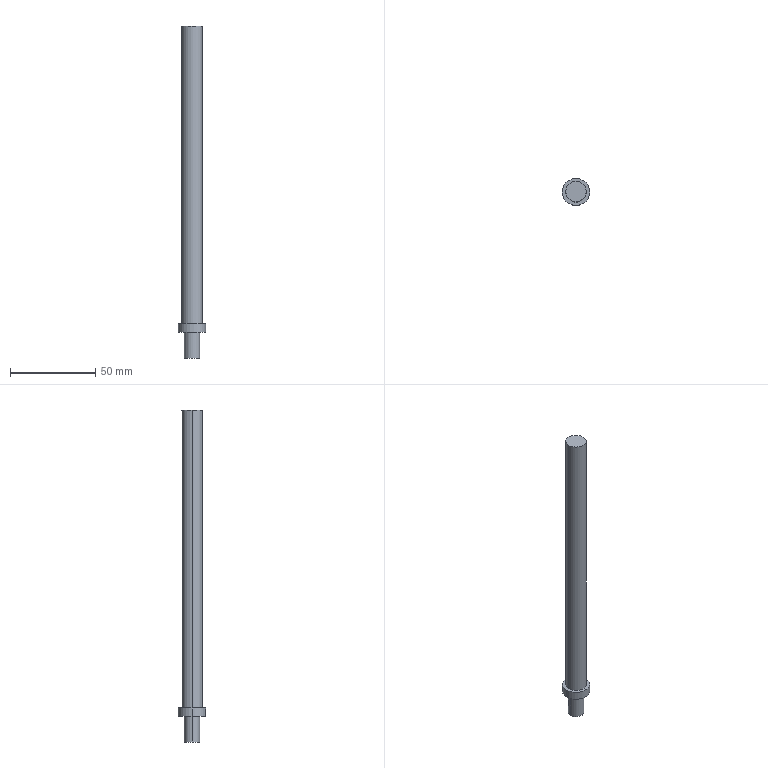Part | SolidWorks | features ICE 2, Extrusion 1 | 1 solid | 10 faces | box 16 x 16 x 195 mm | volume 21752 mm3 | cylinder 6 | plane 4 | commonest cylinder face diameters 9 x2 12 x2 16 x2
STEP:
#1=CARTESIAN_POINT('',(6.,0.,195.));
#2=VERTEX_POINT('',#1);
#3=CARTESIAN_POINT('',(-6.,0.,195.));
#4=VERTEX_POINT('',#3);
#5=CARTESIAN_POINT('',(0.,0.,195.));
#6=DIRECTION('',(0.,0.,1.));
#7=DIRECTION('',(1.,0.,0.));
#8=AXIS2_PLACEMENT_3D('',#5,#6,#7);
#9=CIRCLE('',#8,6.);
#10=EDGE_CURVE('',#2,#4,#9,.T.);
#11=ORIENTED_EDGE('',*,*,#10,.F.);
#12=CARTESIAN_POINT('',(6.,0.,20.));
#13=VERTEX_POINT('',#12);
#14=CARTESIAN_POINT('',(6.,0.,195.));
#15=DIRECTION('',(0.,0.,-1.));
#16=VECTOR('',#15,1000.);
#17=LINE('',#14,#16);
#18=EDGE_CURVE('',#2,#13,#17,.T.);
#19=ORIENTED_EDGE('',*,*,#18,.T.);
#20=CARTESIAN_POINT('',(-6.,0.,20.));
#21=VERTEX_POINT('',#20);
#22=CARTESIAN_POINT('',(0.,0.,20.));
#23=DIRECTION('',(0.,0.,-1.));
#24=DIRECTION('',(-1.,0.,0.));
#25=AXIS2_PLACEMENT_3D('',#22,#23,#24);
#26=CIRCLE('',#25,6.);
#27=EDGE_CURVE('',#21,#13,#26,.T.);
#28=ORIENTED_EDGE('',*,*,#27,.F.);
#29=CARTESIAN_POINT('',(-6.,0.,195.));
#30=DIRECTION('',(0.,0.,-1.));
#31=VECTOR('',#30,1000.);
#32=LINE('',#29,#31);
#33=EDGE_CURVE('',#4,#21,#32,.T.);
#34=ORIENTED_EDGE('',*,*,#33,.F.);
#35=EDGE_LOOP('',(#11,#19,#28,#34));
#36=FACE_OUTER_BOUND('',#35,.T.);
#37=CARTESIAN_POINT('',(0.,0.,195.));
#38=DIRECTION('',(0.,0.,-1.));
#39=DIRECTION('',(-1.,0.,0.));
#40=AXIS2_PLACEMENT_3D('',#37,#38,#39);
#41=CYLINDRICAL_SURFACE('',#40,6.);
#42=ADVANCED_FACE('',(#36),#41,.T.);
#43=CARTESIAN_POINT('',(-8.,0.,20.));
#44=VERTEX_POINT('',#43);
#45=CARTESIAN_POINT('',(8.,0.,20.));
#46=VERTEX_POINT('',#45);
#47=CARTESIAN_POINT('',(0.,0.,20.));
#48=DIRECTION('',(0.,0.,-1.));
#49=DIRECTION('',(-1.,0.,0.));
#50=AXIS2_PLACEMENT_3D('',#47,#48,#49);
#51=CIRCLE('',#50,8.);
#52=EDGE_CURVE('',#44,#46,#51,.T.);
#53=ORIENTED_EDGE('',*,*,#52,.T.);
#54=CARTESIAN_POINT('',(8.,0.,15.));
#55=VERTEX_POINT('',#54);
#56=CARTESIAN_POINT('',(8.,0.,20.));
#57=DIRECTION('',(0.,0.,-1.));
#58=VECTOR('',#57,1000.);
#59=LINE('',#56,#58);
#60=EDGE_CURVE('',#46,#55,#59,.T.);
#61=ORIENTED_EDGE('',*,*,#60,.T.);
#62=CARTESIAN_POINT('',(-8.,0.,15.));
#63=VERTEX_POINT('',#62);
#64=CARTESIAN_POINT('',(0.,0.,15.));
#65=DIRECTION('',(0.,0.,-1.));
#66=DIRECTION('',(-1.,0.,0.));
#67=AXIS2_PLACEMENT_3D('',#64,#65,#66);
#68=CIRCLE('',#67,8.);
#69=EDGE_CURVE('',#63,#55,#68,.T.);
#70=ORIENTED_EDGE('',*,*,#69,.F.);
#71=CARTESIAN_POINT('',(-8.,0.,20.));
#72=DIRECTION('',(0.,0.,-1.));
#73=VECTOR('',#72,1000.);
#74=LINE('',#71,#73);
#75=EDGE_CURVE('',#44,#63,#74,.T.);
#76=ORIENTED_EDGE('',*,*,#75,.F.);
#77=EDGE_LOOP('',(#53,#61,#70,#76));
#78=FACE_OUTER_BOUND('',#77,.T.);
#79=CARTESIAN_POINT('',(0.,0.,20.));
#80=DIRECTION('',(0.,0.,-1.));
#81=DIRECTION('',(-1.,0.,0.));
#82=AXIS2_PLACEMENT_3D('',#79,#80,#81);
#83=CYLINDRICAL_SURFACE('',#82,8.);
#84=ADVANCED_FACE('',(#78),#83,.T.);
#85=CARTESIAN_POINT('',(4.5,0.,15.));
#86=VERTEX_POINT('',#85);
#87=CARTESIAN_POINT('',(-4.5,0.,15.));
#88=VERTEX_POINT('',#87);
#89=CARTESIAN_POINT('',(0.,0.,15.));
#90=DIRECTION('',(0.,0.,1.));
#91=DIRECTION('',(1.,0.,0.));
#92=AXIS2_PLACEMENT_3D('',#89,#90,#91);
#93=CIRCLE('',#92,4.5);
#94=EDGE_CURVE('',#86,#88,#93,.T.);
#95=ORIENTED_EDGE('',*,*,#94,.F.);
#96=CARTESIAN_POINT('',(4.5,0.,0.));
#97=VERTEX_POINT('',#96);
#98=CARTESIAN_POINT('',(4.5,0.,15.));
#99=DIRECTION('',(0.,0.,-1.));
#100=VECTOR('',#99,1000.);
#101=LINE('',#98,#100);
#102=EDGE_CURVE('',#86,#97,#101,.T.);
#103=ORIENTED_EDGE('',*,*,#102,.T.);
#104=CARTESIAN_POINT('',(-4.5,0.,0.));
#105=VERTEX_POINT('',#104);
#106=CARTESIAN_POINT('',(0.,0.,0.));
#107=DIRECTION('',(0.,0.,1.));
#108=DIRECTION('',(1.,0.,0.));
#109=AXIS2_PLACEMENT_3D('',#106,#107,#108);
#110=CIRCLE('',#109,4.5);
#111=EDGE_CURVE('',#97,#105,#110,.T.);
#112=ORIENTED_EDGE('',*,*,#111,.T.);
#113=CARTESIAN_POINT('',(-4.5,0.,15.));
#114=DIRECTION('',(0.,0.,-1.));
#115=VECTOR('',#114,1000.);
#116=LINE('',#113,#115);
#117=EDGE_CURVE('',#88,#105,#116,.T.);
#118=ORIENTED_EDGE('',*,*,#117,.F.);
#119=EDGE_LOOP('',(#95,#103,#112,#118));
#120=FACE_OUTER_BOUND('',#119,.T.);
#121=CARTESIAN_POINT('',(0.,0.,15.));
#122=DIRECTION('',(0.,0.,-1.));
#123=DIRECTION('',(-1.,0.,0.));
#124=AXIS2_PLACEMENT_3D('',#121,#122,#123);
#125=CYLINDRICAL_SURFACE('',#124,4.5);
#126=ADVANCED_FACE('',(#120),#125,.T.);
#127=ORIENTED_EDGE('',*,*,#102,.F.);
#128=CARTESIAN_POINT('',(0.,0.,15.));
#129=DIRECTION('',(0.,0.,1.));
#130=DIRECTION('',(1.,0.,0.));
#131=AXIS2_PLACEMENT_3D('',#128,#129,#130);
#132=CIRCLE('',#131,4.5);
#133=EDGE_CURVE('',#88,#86,#132,.T.);
#134=ORIENTED_EDGE('',*,*,#133,.F.);
#135=ORIENTED_EDGE('',*,*,#117,.T.);
#136=CARTESIAN_POINT('',(0.,0.,0.));
#137=DIRECTION('',(0.,0.,1.));
#138=DIRECTION('',(1.,0.,0.));
#139=AXIS2_PLACEMENT_3D('',#136,#137,#138);
#140=CIRCLE('',#139,4.5);
#141=EDGE_CURVE('',#105,#97,#140,.T.);
#142=ORIENTED_EDGE('',*,*,#141,.T.);
#143=EDGE_LOOP('',(#127,#134,#135,#142));
#144=FACE_OUTER_BOUND('',#143,.T.);
#145=CARTESIAN_POINT('',(0.,0.,15.));
#146=DIRECTION('',(0.,0.,-1.));
#147=DIRECTION('',(-1.,0.,0.));
#148=AXIS2_PLACEMENT_3D('',#145,#146,#147);
#149=CYLINDRICAL_SURFACE('',#148,4.5);
#150=ADVANCED_FACE('',(#144),#149,.T.);
#151=ORIENTED_EDGE('',*,*,#141,.F.);
#152=ORIENTED_EDGE('',*,*,#111,.F.);
#153=EDGE_LOOP('',(#151,#152));
#154=FACE_OUTER_BOUND('',#153,.T.);
#155=CARTESIAN_POINT('',(0.,0.,0.));
#156=DIRECTION('',(0.,0.,1.));
#157=DIRECTION('',(1.,0.,0.));
#158=AXIS2_PLACEMENT_3D('',#155,#156,#157);
#159=PLANE('',#158);
#160=ADVANCED_FACE('',(#154),#159,.F.);
#161=ORIENTED_EDGE('',*,*,#133,.T.);
#162=ORIENTED_EDGE('',*,*,#94,.T.);
#163=EDGE_LOOP('',(#161,#162));
#164=FACE_BOUND('',#163,.T.);
#165=ORIENTED_EDGE('',*,*,#69,.T.);
#166=CARTESIAN_POINT('',(0.,0.,15.));
#167=DIRECTION('',(0.,0.,-1.));
#168=DIRECTION('',(-1.,0.,0.));
#169=AXIS2_PLACEMENT_3D('',#166,#167,#168);
#170=CIRCLE('',#169,8.);
#171=EDGE_CURVE('',#55,#63,#170,.T.);
#172=ORIENTED_EDGE('',*,*,#171,.T.);
#173=EDGE_LOOP('',(#165,#172));
#174=FACE_OUTER_BOUND('',#173,.T.);
#175=CARTESIAN_POINT('',(0.,0.,15.));
#176=DIRECTION('',(0.,0.,1.));
#177=DIRECTION('',(1.,0.,0.));
#178=AXIS2_PLACEMENT_3D('',#175,#176,#177);
#179=PLANE('',#178);
#180=ADVANCED_FACE('',(#164,#174),#179,.F.);
#181=ORIENTED_EDGE('',*,*,#60,.F.);
#182=CARTESIAN_POINT('',(0.,0.,20.));
#183=DIRECTION('',(0.,0.,-1.));
#184=DIRECTION('',(-1.,0.,0.));
#185=AXIS2_PLACEMENT_3D('',#182,#183,#184);
#186=CIRCLE('',#185,8.);
#187=EDGE_CURVE('',#46,#44,#186,.T.);
#188=ORIENTED_EDGE('',*,*,#187,.T.);
#189=ORIENTED_EDGE('',*,*,#75,.T.);
#190=ORIENTED_EDGE('',*,*,#171,.F.);
#191=EDGE_LOOP('',(#181,#188,#189,#190));
#192=FACE_OUTER_BOUND('',#191,.T.);
#193=CARTESIAN_POINT('',(0.,0.,20.));
#194=DIRECTION('',(0.,0.,-1.));
#195=DIRECTION('',(-1.,0.,0.));
#196=AXIS2_PLACEMENT_3D('',#193,#194,#195);
#197=CYLINDRICAL_SURFACE('',#196,8.);
#198=ADVANCED_FACE('',(#192),#197,.T.);
#199=ORIENTED_EDGE('',*,*,#27,.T.);
#200=CARTESIAN_POINT('',(0.,0.,20.));
#201=DIRECTION('',(0.,0.,-1.));
#202=DIRECTION('',(-1.,0.,0.));
#203=AXIS2_PLACEMENT_3D('',#200,#201,#202);
#204=CIRCLE('',#203,6.);
#205=EDGE_CURVE('',#13,#21,#204,.T.);
#206=ORIENTED_EDGE('',*,*,#205,.T.);
#207=EDGE_LOOP('',(#199,#206));
#208=FACE_BOUND('',#207,.T.);
#209=ORIENTED_EDGE('',*,*,#52,.F.);
#210=ORIENTED_EDGE('',*,*,#187,.F.);
#211=EDGE_LOOP('',(#209,#210));
#212=FACE_OUTER_BOUND('',#211,.T.);
#213=CARTESIAN_POINT('',(0.,0.,20.));
#214=DIRECTION('',(0.,0.,-1.));
#215=DIRECTION('',(-1.,0.,0.));
#216=AXIS2_PLACEMENT_3D('',#213,#214,#215);
#217=PLANE('',#216);
#218=ADVANCED_FACE('',(#208,#212),#217,.F.);
#219=CARTESIAN_POINT('',(0.,0.,195.));
#220=DIRECTION('',(0.,0.,1.));
#221=DIRECTION('',(1.,0.,0.));
#222=AXIS2_PLACEMENT_3D('',#219,#220,#221);
#223=CIRCLE('',#222,6.);
#224=EDGE_CURVE('',#4,#2,#223,.T.);
#225=ORIENTED_EDGE('',*,*,#224,.T.);
#226=ORIENTED_EDGE('',*,*,#10,.T.);
#227=EDGE_LOOP('',(#225,#226));
#228=FACE_OUTER_BOUND('',#227,.T.);
#229=CARTESIAN_POINT('',(0.,0.,195.));
#230=DIRECTION('',(0.,0.,1.));
#231=DIRECTION('',(1.,0.,0.));
#232=AXIS2_PLACEMENT_3D('',#229,#230,#231);
#233=PLANE('',#232);
#234=ADVANCED_FACE('',(#228),#233,.T.);
#235=ORIENTED_EDGE('',*,*,#18,.F.);
#236=ORIENTED_EDGE('',*,*,#224,.F.);
#237=ORIENTED_EDGE('',*,*,#33,.T.);
#238=ORIENTED_EDGE('',*,*,#205,.F.);
#239=EDGE_LOOP('',(#235,#236,#237,#238));
#240=FACE_OUTER_BOUND('',#239,.T.);
#241=CARTESIAN_POINT('',(0.,0.,195.));
#242=DIRECTION('',(0.,0.,-1.));
#243=DIRECTION('',(-1.,0.,0.));
#244=AXIS2_PLACEMENT_3D('',#241,#242,#243);
#245=CYLINDRICAL_SURFACE('',#244,6.);
#246=ADVANCED_FACE('',(#240),#245,.T.);
#247=CLOSED_SHELL('',(#42,#84,#126,#150,#160,#180,#198,#218,#234,#246));
#248=MANIFOLD_SOLID_BREP('',#247);
#249=CARTESIAN_POINT('',(0.,0.,0.));
#250=DIRECTION('',(0.,0.,1.));
#251=DIRECTION('',(1.,0.,0.));
#252=AXIS2_PLACEMENT_3D('',#249,#250,#251);
#253=(LENGTH_UNIT()NAMED_UNIT(*)SI_UNIT(.MILLI.,.METRE.));
#254=UNCERTAINTY_MEASURE_WITH_UNIT(LENGTH_MEASURE(0.00001),#253,'','');
#255=(NAMED_UNIT(*)PLANE_ANGLE_UNIT()SI_UNIT($,.RADIAN.));
#256=(NAMED_UNIT(*)SI_UNIT($,.STERADIAN.)SOLID_ANGLE_UNIT());
#257=(GEOMETRIC_REPRESENTATION_CONTEXT(3)GLOBAL_UNCERTAINTY_ASSIGNED_CONTEXT((#254))GLOBAL_UNIT_ASSIGNED_CONTEXT((#253,#255,#256))REPRESENTATION_CONTEXT('',''));
#258=ADVANCED_BREP_SHAPE_REPRESENTATION('',(#248,#252),#257);